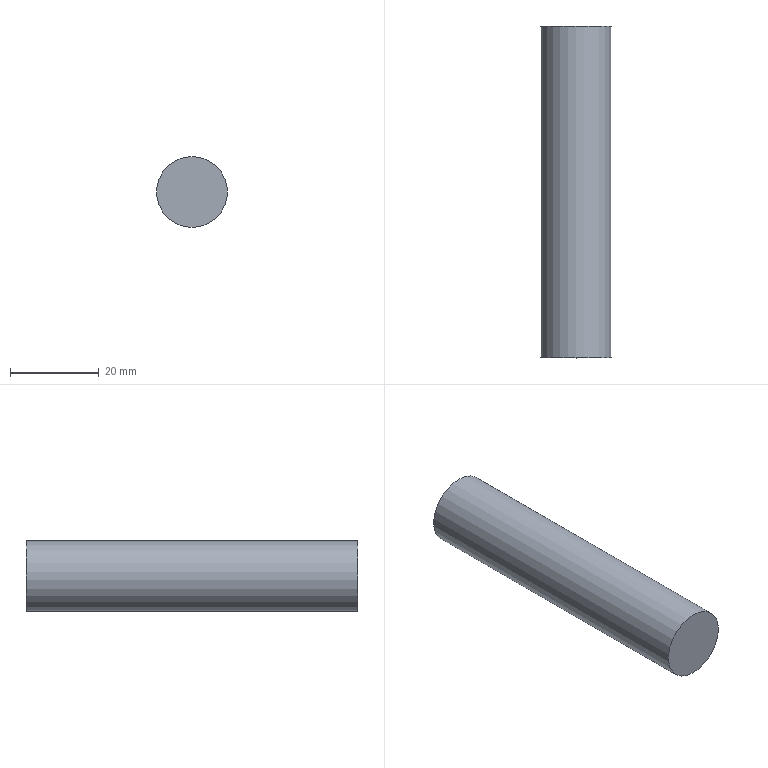Part | STEP file | solid 164 | 1 solid | 3 faces | box 16 x 75 x 16 mm | volume 15080 mm3 | plane 2 | cylinder 1 | commonest cylinder face diameters 16 x1